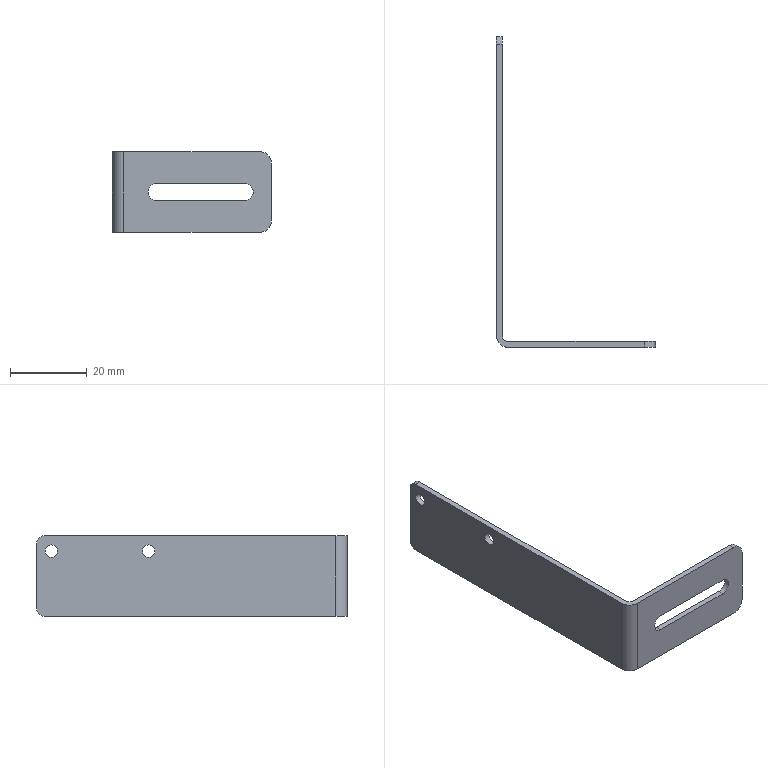Part | STEP file | ROTATION MC_NEW VER-0610_516 | 1 solid | 20 faces | box 41.5 x 81.002 x 21 mm | volume 3574 mm3 | plane 10 | cylinder 10 | commonest cylinder face diameters 6 x3 3.2 x2 4 x2 4.4 x2 3 x1
STEP:
#1=CARTESIAN_POINT('',(-92.489,288.968,-73.528));
#2=VERTEX_POINT('',#1);
#3=CARTESIAN_POINT('',(-115.489,288.968,-73.528));
#4=VERTEX_POINT('',#3);
#5=CARTESIAN_POINT('',(-121.239,288.968,-73.528));
#6=DIRECTION('',(-1.,0.,0.));
#7=VECTOR('',#6,10.);
#8=LINE('',#5,#7);
#9=EDGE_CURVE('',#2,#4,#8,.T.);
#10=ORIENTED_EDGE('',*,*,#9,.F.);
#11=CARTESIAN_POINT('',(-92.489,290.468,-73.528));
#12=VERTEX_POINT('',#11);
#13=CARTESIAN_POINT('',(-92.489,290.468,-73.528));
#14=DIRECTION('',(0.,-1.,0.));
#15=VECTOR('',#14,10.);
#16=LINE('',#13,#15);
#17=EDGE_CURVE('',#12,#2,#16,.T.);
#18=ORIENTED_EDGE('',*,*,#17,.F.);
#19=CARTESIAN_POINT('',(-115.489,290.468,-73.528));
#20=VERTEX_POINT('',#19);
#21=CARTESIAN_POINT('',(-120.489,290.468,-73.528));
#22=DIRECTION('',(1.,0.,0.));
#23=VECTOR('',#22,10.);
#24=LINE('',#21,#23);
#25=EDGE_CURVE('',#20,#12,#24,.T.);
#26=ORIENTED_EDGE('',*,*,#25,.F.);
#27=CARTESIAN_POINT('',(-115.489,290.468,-73.528));
#28=DIRECTION('',(0.,-1.,0.));
#29=VECTOR('',#28,10.);
#30=LINE('',#27,#29);
#31=EDGE_CURVE('',#20,#4,#30,.T.);
#32=ORIENTED_EDGE('',*,*,#31,.T.);
#33=EDGE_LOOP('',(#10,#18,#26,#32));
#34=FACE_OUTER_BOUND('',#33,.T.);
#35=CARTESIAN_POINT('',(-115.489,290.468,-73.528));
#36=DIRECTION('',(0.,0.,-1.));
#37=DIRECTION('',(1.,0.,0.));
#38=AXIS2_PLACEMENT_3D('',#35,#36,#37);
#39=PLANE('',#38);
#40=ADVANCED_FACE('',(#34),#39,.F.);
#41=CARTESIAN_POINT('',(-115.489,288.968,-69.128));
#42=VERTEX_POINT('',#41);
#43=CARTESIAN_POINT('',(-115.489,288.968,-71.328));
#44=DIRECTION('',(0.,1.,0.));
#45=DIRECTION('',(0.,0.,-1.));
#46=AXIS2_PLACEMENT_3D('',#43,#44,#45);
#47=CIRCLE('',#46,2.2);
#48=EDGE_CURVE('',#4,#42,#47,.T.);
#49=ORIENTED_EDGE('',*,*,#48,.F.);
#50=ORIENTED_EDGE('',*,*,#31,.F.);
#51=CARTESIAN_POINT('',(-115.489,290.468,-69.128));
#52=VERTEX_POINT('',#51);
#53=CARTESIAN_POINT('',(-115.489,290.468,-71.328));
#54=DIRECTION('',(0.,-1.,0.));
#55=DIRECTION('',(0.,0.,-1.));
#56=AXIS2_PLACEMENT_3D('',#53,#54,#55);
#57=CIRCLE('',#56,2.2);
#58=EDGE_CURVE('',#52,#20,#57,.T.);
#59=ORIENTED_EDGE('',*,*,#58,.F.);
#60=CARTESIAN_POINT('',(-115.489,290.468,-69.128));
#61=DIRECTION('',(0.,-1.,0.));
#62=VECTOR('',#61,10.);
#63=LINE('',#60,#62);
#64=EDGE_CURVE('',#52,#42,#63,.T.);
#65=ORIENTED_EDGE('',*,*,#64,.T.);
#66=EDGE_LOOP('',(#49,#50,#59,#65));
#67=FACE_OUTER_BOUND('',#66,.T.);
#68=CARTESIAN_POINT('',(-115.489,290.468,-71.328));
#69=DIRECTION('',(0.,-1.,0.));
#70=DIRECTION('',(0.,0.,-1.));
#71=AXIS2_PLACEMENT_3D('',#68,#69,#70);
#72=CYLINDRICAL_SURFACE('',#71,2.2);
#73=ADVANCED_FACE('',(#67),#72,.F.);
#74=CARTESIAN_POINT('',(-92.489,288.968,-69.128));
#75=VERTEX_POINT('',#74);
#76=CARTESIAN_POINT('',(-109.739,288.968,-69.128));
#77=DIRECTION('',(1.,0.,0.));
#78=VECTOR('',#77,10.);
#79=LINE('',#76,#78);
#80=EDGE_CURVE('',#42,#75,#79,.T.);
#81=ORIENTED_EDGE('',*,*,#80,.F.);
#82=ORIENTED_EDGE('',*,*,#64,.F.);
#83=CARTESIAN_POINT('',(-92.489,290.468,-69.128));
#84=VERTEX_POINT('',#83);
#85=CARTESIAN_POINT('',(-108.989,290.468,-69.128));
#86=DIRECTION('',(-1.,0.,0.));
#87=VECTOR('',#86,10.);
#88=LINE('',#85,#87);
#89=EDGE_CURVE('',#84,#52,#88,.T.);
#90=ORIENTED_EDGE('',*,*,#89,.F.);
#91=CARTESIAN_POINT('',(-92.489,290.468,-69.128));
#92=DIRECTION('',(0.,-1.,0.));
#93=VECTOR('',#92,10.);
#94=LINE('',#91,#93);
#95=EDGE_CURVE('',#84,#75,#94,.T.);
#96=ORIENTED_EDGE('',*,*,#95,.T.);
#97=EDGE_LOOP('',(#81,#82,#90,#96));
#98=FACE_OUTER_BOUND('',#97,.T.);
#99=CARTESIAN_POINT('',(-92.489,290.468,-69.128));
#100=DIRECTION('',(0.,0.,1.));
#101=DIRECTION('',(-1.,0.,0.));
#102=AXIS2_PLACEMENT_3D('',#99,#100,#101);
#103=PLANE('',#102);
#104=ADVANCED_FACE('',(#98),#103,.F.);
#105=CARTESIAN_POINT('',(-92.489,288.968,-71.328));
#106=DIRECTION('',(0.,1.,0.));
#107=DIRECTION('',(0.,0.,1.));
#108=AXIS2_PLACEMENT_3D('',#105,#106,#107);
#109=CIRCLE('',#108,2.2);
#110=EDGE_CURVE('',#75,#2,#109,.T.);
#111=ORIENTED_EDGE('',*,*,#110,.F.);
#112=ORIENTED_EDGE('',*,*,#95,.F.);
#113=CARTESIAN_POINT('',(-92.489,290.468,-71.328));
#114=DIRECTION('',(0.,-1.,0.));
#115=DIRECTION('',(0.,0.,1.));
#116=AXIS2_PLACEMENT_3D('',#113,#114,#115);
#117=CIRCLE('',#116,2.2);
#118=EDGE_CURVE('',#12,#84,#117,.T.);
#119=ORIENTED_EDGE('',*,*,#118,.F.);
#120=ORIENTED_EDGE('',*,*,#17,.T.);
#121=EDGE_LOOP('',(#111,#112,#119,#120));
#122=FACE_OUTER_BOUND('',#121,.T.);
#123=CARTESIAN_POINT('',(-92.489,290.468,-71.328));
#124=DIRECTION('',(0.,-1.,0.));
#125=DIRECTION('',(0.,0.,1.));
#126=AXIS2_PLACEMENT_3D('',#123,#124,#125);
#127=CYLINDRICAL_SURFACE('',#126,2.2);
#128=ADVANCED_FACE('',(#122),#127,.F.);
#129=CARTESIAN_POINT('',(-88.489,290.468,-81.828));
#130=VERTEX_POINT('',#129);
#131=CARTESIAN_POINT('',(-85.489,290.468,-78.828));
#132=VERTEX_POINT('',#131);
#133=CARTESIAN_POINT('',(-88.489,290.468,-78.828));
#134=DIRECTION('',(0.,-1.,0.));
#135=DIRECTION('',(0.7071,0.,-0.7071));
#136=AXIS2_PLACEMENT_3D('',#133,#134,#135);
#137=CIRCLE('',#136,3.);
#138=EDGE_CURVE('',#130,#132,#137,.T.);
#139=ORIENTED_EDGE('',*,*,#138,.T.);
#140=CARTESIAN_POINT('',(-85.489,288.968,-78.828));
#141=VERTEX_POINT('',#140);
#142=CARTESIAN_POINT('',(-85.489,386.581,-78.828));
#143=DIRECTION('',(0.,-1.,0.));
#144=VECTOR('',#143,10.);
#145=LINE('',#142,#144);
#146=EDGE_CURVE('',#132,#141,#145,.T.);
#147=ORIENTED_EDGE('',*,*,#146,.T.);
#148=CARTESIAN_POINT('',(-88.489,288.968,-81.828));
#149=VERTEX_POINT('',#148);
#150=CARTESIAN_POINT('',(-88.489,288.968,-78.828));
#151=DIRECTION('',(0.,1.,0.));
#152=DIRECTION('',(0.7071,0.,-0.7071));
#153=AXIS2_PLACEMENT_3D('',#150,#151,#152);
#154=CIRCLE('',#153,3.);
#155=EDGE_CURVE('',#141,#149,#154,.T.);
#156=ORIENTED_EDGE('',*,*,#155,.T.);
#157=CARTESIAN_POINT('',(-88.489,386.581,-81.828));
#158=DIRECTION('',(0.,1.,0.));
#159=VECTOR('',#158,10.);
#160=LINE('',#157,#159);
#161=EDGE_CURVE('',#149,#130,#160,.T.);
#162=ORIENTED_EDGE('',*,*,#161,.T.);
#163=EDGE_LOOP('',(#139,#147,#156,#162));
#164=FACE_OUTER_BOUND('',#163,.T.);
#165=CARTESIAN_POINT('',(-88.489,386.581,-78.828));
#166=DIRECTION('',(0.,1.,0.));
#167=DIRECTION('',(0.7071,0.,-0.7071));
#168=AXIS2_PLACEMENT_3D('',#165,#166,#167);
#169=CYLINDRICAL_SURFACE('',#168,3.);
#170=ADVANCED_FACE('',(#164),#169,.T.);
#171=ORIENTED_EDGE('',*,*,#155,.F.);
#172=CARTESIAN_POINT('',(-85.489,288.968,-63.828));
#173=VERTEX_POINT('',#172);
#174=CARTESIAN_POINT('',(-85.489,288.968,-78.828));
#175=DIRECTION('',(0.,0.,1.));
#176=VECTOR('',#175,15.);
#177=LINE('',#174,#176);
#178=EDGE_CURVE('',#141,#173,#177,.T.);
#179=ORIENTED_EDGE('',*,*,#178,.T.);
#180=CARTESIAN_POINT('',(-88.489,288.968,-60.828));
#181=VERTEX_POINT('',#180);
#182=CARTESIAN_POINT('',(-88.489,288.968,-63.828));
#183=DIRECTION('',(0.,1.,0.));
#184=DIRECTION('',(0.7071,0.,0.7071));
#185=AXIS2_PLACEMENT_3D('',#182,#183,#184);
#186=CIRCLE('',#185,3.);
#187=EDGE_CURVE('',#181,#173,#186,.T.);
#188=ORIENTED_EDGE('',*,*,#187,.F.);
#189=CARTESIAN_POINT('',(-123.989,288.968,-60.828));
#190=VERTEX_POINT('',#189);
#191=CARTESIAN_POINT('',(-123.989,288.968,-60.828));
#192=DIRECTION('',(1.,0.,0.));
#193=VECTOR('',#192,25.5);
#194=LINE('',#191,#193);
#195=EDGE_CURVE('',#190,#181,#194,.T.);
#196=ORIENTED_EDGE('',*,*,#195,.F.);
#197=CARTESIAN_POINT('',(-123.989,288.968,-81.828));
#198=VERTEX_POINT('',#197);
#199=CARTESIAN_POINT('',(-123.989,288.968,-81.828));
#200=DIRECTION('',(0.,0.,1.));
#201=VECTOR('',#200,21.);
#202=LINE('',#199,#201);
#203=EDGE_CURVE('',#198,#190,#202,.T.);
#204=ORIENTED_EDGE('',*,*,#203,.F.);
#205=CARTESIAN_POINT('',(-123.989,288.968,-81.828));
#206=DIRECTION('',(1.,0.,0.));
#207=VECTOR('',#206,25.5);
#208=LINE('',#205,#207);
#209=EDGE_CURVE('',#198,#149,#208,.T.);
#210=ORIENTED_EDGE('',*,*,#209,.T.);
#211=EDGE_LOOP('',(#171,#179,#188,#196,#204,#210));
#212=FACE_OUTER_BOUND('',#211,.T.);
#213=ORIENTED_EDGE('',*,*,#80,.T.);
#214=ORIENTED_EDGE('',*,*,#110,.T.);
#215=ORIENTED_EDGE('',*,*,#9,.T.);
#216=ORIENTED_EDGE('',*,*,#48,.T.);
#217=EDGE_LOOP('',(#213,#214,#215,#216));
#218=FACE_BOUND('',#217,.T.);
#219=CARTESIAN_POINT('',(-126.989,288.968,-71.591));
#220=DIRECTION('',(0.,-1.,0.));
#221=DIRECTION('',(0.,0.,-1.));
#222=AXIS2_PLACEMENT_3D('',#219,#220,#221);
#223=PLANE('',#222);
#224=ADVANCED_FACE('',(#212,#218),#223,.T.);
#225=ORIENTED_EDGE('',*,*,#146,.F.);
#226=CARTESIAN_POINT('',(-85.489,290.468,-63.828));
#227=VERTEX_POINT('',#226);
#228=CARTESIAN_POINT('',(-85.489,290.468,-78.828));
#229=DIRECTION('',(0.,0.,1.));
#230=VECTOR('',#229,15.);
#231=LINE('',#228,#230);
#232=EDGE_CURVE('',#132,#227,#231,.T.);
#233=ORIENTED_EDGE('',*,*,#232,.T.);
#234=CARTESIAN_POINT('',(-85.489,386.581,-63.828));
#235=DIRECTION('',(0.,1.,0.));
#236=VECTOR('',#235,10.);
#237=LINE('',#234,#236);
#238=EDGE_CURVE('',#173,#227,#237,.T.);
#239=ORIENTED_EDGE('',*,*,#238,.F.);
#240=ORIENTED_EDGE('',*,*,#178,.F.);
#241=EDGE_LOOP('',(#225,#233,#239,#240));
#242=FACE_OUTER_BOUND('',#241,.T.);
#243=CARTESIAN_POINT('',(-85.489,422.081,-91.591));
#244=DIRECTION('',(1.,0.,0.));
#245=DIRECTION('',(0.,0.,-1.));
#246=AXIS2_PLACEMENT_3D('',#243,#244,#245);
#247=PLANE('',#246);
#248=ADVANCED_FACE('',(#242),#247,.T.);
#249=CARTESIAN_POINT('',(-88.489,290.468,-60.828));
#250=VERTEX_POINT('',#249);
#251=CARTESIAN_POINT('',(-88.489,290.468,-63.828));
#252=DIRECTION('',(0.,-1.,0.));
#253=DIRECTION('',(0.7071,0.,0.7071));
#254=AXIS2_PLACEMENT_3D('',#251,#252,#253);
#255=CIRCLE('',#254,3.);
#256=EDGE_CURVE('',#227,#250,#255,.T.);
#257=ORIENTED_EDGE('',*,*,#256,.T.);
#258=CARTESIAN_POINT('',(-88.489,386.581,-60.828));
#259=DIRECTION('',(0.,-1.,0.));
#260=VECTOR('',#259,10.);
#261=LINE('',#258,#260);
#262=EDGE_CURVE('',#250,#181,#261,.T.);
#263=ORIENTED_EDGE('',*,*,#262,.T.);
#264=ORIENTED_EDGE('',*,*,#187,.T.);
#265=ORIENTED_EDGE('',*,*,#238,.T.);
#266=EDGE_LOOP('',(#257,#263,#264,#265));
#267=FACE_OUTER_BOUND('',#266,.T.);
#268=CARTESIAN_POINT('',(-88.489,386.581,-63.828));
#269=DIRECTION('',(0.,1.,0.));
#270=DIRECTION('',(0.7071,0.,0.7071));
#271=AXIS2_PLACEMENT_3D('',#268,#269,#270);
#272=CYLINDRICAL_SURFACE('',#271,3.);
#273=ADVANCED_FACE('',(#267),#272,.T.);
#274=ORIENTED_EDGE('',*,*,#161,.F.);
#275=ORIENTED_EDGE('',*,*,#209,.F.);
#276=CARTESIAN_POINT('',(-126.989,291.968,-81.828));
#277=VERTEX_POINT('',#276);
#278=CARTESIAN_POINT('',(-123.989,291.968,-81.828));
#279=DIRECTION('',(0.,0.,1.));
#280=DIRECTION('',(-0.7071,-0.7071,0.));
#281=AXIS2_PLACEMENT_3D('',#278,#279,#280);
#282=CIRCLE('',#281,3.);
#283=EDGE_CURVE('',#277,#198,#282,.T.);
#284=ORIENTED_EDGE('',*,*,#283,.F.);
#285=CARTESIAN_POINT('',(-126.989,367.967,-81.828));
#286=VERTEX_POINT('',#285);
#287=CARTESIAN_POINT('',(-126.989,367.967,-81.828));
#288=DIRECTION('',(0.,-1.,0.));
#289=VECTOR('',#288,75.999);
#290=LINE('',#287,#289);
#291=EDGE_CURVE('',#286,#277,#290,.T.);
#292=ORIENTED_EDGE('',*,*,#291,.F.);
#293=CARTESIAN_POINT('',(-125.489,367.967,-81.828));
#294=VERTEX_POINT('',#293);
#295=CARTESIAN_POINT('',(-126.989,367.967,-81.828));
#296=DIRECTION('',(1.,0.,0.));
#297=VECTOR('',#296,1.5);
#298=LINE('',#295,#297);
#299=EDGE_CURVE('',#286,#294,#298,.T.);
#300=ORIENTED_EDGE('',*,*,#299,.T.);
#301=CARTESIAN_POINT('',(-125.489,291.968,-81.828));
#302=VERTEX_POINT('',#301);
#303=CARTESIAN_POINT('',(-125.489,367.967,-81.828));
#304=DIRECTION('',(0.,-1.,0.));
#305=VECTOR('',#304,75.999);
#306=LINE('',#303,#305);
#307=EDGE_CURVE('',#294,#302,#306,.T.);
#308=ORIENTED_EDGE('',*,*,#307,.T.);
#309=CARTESIAN_POINT('',(-123.989,290.468,-81.828));
#310=VERTEX_POINT('',#309);
#311=CARTESIAN_POINT('',(-123.989,291.968,-81.828));
#312=DIRECTION('',(0.,0.,-1.));
#313=DIRECTION('',(-0.7071,-0.7071,0.));
#314=AXIS2_PLACEMENT_3D('',#311,#312,#313);
#315=CIRCLE('',#314,1.5);
#316=EDGE_CURVE('',#310,#302,#315,.T.);
#317=ORIENTED_EDGE('',*,*,#316,.F.);
#318=CARTESIAN_POINT('',(-98.489,290.468,-81.828));
#319=DIRECTION('',(-1.,0.,0.));
#320=VECTOR('',#319,25.5);
#321=LINE('',#318,#320);
#322=EDGE_CURVE('',#130,#310,#321,.T.);
#323=ORIENTED_EDGE('',*,*,#322,.F.);
#324=EDGE_LOOP('',(#274,#275,#284,#292,#300,#308,#317,#323));
#325=FACE_OUTER_BOUND('',#324,.T.);
#326=CARTESIAN_POINT('',(-126.989,351.081,-81.828));
#327=DIRECTION('',(0.,0.,-1.));
#328=DIRECTION('',(-1.,0.,0.));
#329=AXIS2_PLACEMENT_3D('',#326,#327,#328);
#330=PLANE('',#329);
#331=ADVANCED_FACE('',(#325),#330,.T.);
#332=CARTESIAN_POINT('',(-126.989,367.97,-60.828));
#333=VERTEX_POINT('',#332);
#334=CARTESIAN_POINT('',(-126.989,369.97,-62.829));
#335=VERTEX_POINT('',#334);
#336=CARTESIAN_POINT('',(-126.989,367.97,-62.828));
#337=DIRECTION('',(-1.,0.,0.));
#338=DIRECTION('',(0.,0.,-1.));
#339=AXIS2_PLACEMENT_3D('',#336,#337,#338);
#340=CIRCLE('',#339,2.);
#341=EDGE_CURVE('',#333,#335,#340,.T.);
#342=ORIENTED_EDGE('',*,*,#341,.F.);
#343=CARTESIAN_POINT('',(-125.489,367.97,-60.828));
#344=VERTEX_POINT('',#343);
#345=CARTESIAN_POINT('',(-125.489,367.97,-60.828));
#346=DIRECTION('',(-1.,0.,0.));
#347=VECTOR('',#346,1.5);
#348=LINE('',#345,#347);
#349=EDGE_CURVE('',#344,#333,#348,.T.);
#350=ORIENTED_EDGE('',*,*,#349,.F.);
#351=CARTESIAN_POINT('',(-125.489,369.97,-62.829));
#352=VERTEX_POINT('',#351);
#353=CARTESIAN_POINT('',(-125.489,367.97,-62.828));
#354=DIRECTION('',(1.,0.,0.));
#355=DIRECTION('',(0.,0.,-1.));
#356=AXIS2_PLACEMENT_3D('',#353,#354,#355);
#357=CIRCLE('',#356,2.);
#358=EDGE_CURVE('',#352,#344,#357,.T.);
#359=ORIENTED_EDGE('',*,*,#358,.F.);
#360=CARTESIAN_POINT('',(-126.989,369.97,-62.829));
#361=DIRECTION('',(1.,0.,0.));
#362=VECTOR('',#361,1.5);
#363=LINE('',#360,#362);
#364=EDGE_CURVE('',#335,#352,#363,.T.);
#365=ORIENTED_EDGE('',*,*,#364,.F.);
#366=EDGE_LOOP('',(#342,#350,#359,#365));
#367=FACE_OUTER_BOUND('',#366,.T.);
#368=CARTESIAN_POINT('',(-132.189,367.97,-62.828));
#369=DIRECTION('',(1.,0.,0.));
#370=DIRECTION('',(0.,0.,-1.));
#371=AXIS2_PLACEMENT_3D('',#368,#369,#370);
#372=CYLINDRICAL_SURFACE('',#371,2.);
#373=ADVANCED_FACE('',(#367),#372,.T.);
#374=CARTESIAN_POINT('',(-126.989,369.967,-79.829));
#375=VERTEX_POINT('',#374);
#376=CARTESIAN_POINT('',(-126.989,367.967,-79.828));
#377=DIRECTION('',(-1.,0.,0.));
#378=DIRECTION('',(0.,0.,-1.));
#379=AXIS2_PLACEMENT_3D('',#376,#377,#378);
#380=CIRCLE('',#379,2.);
#381=EDGE_CURVE('',#375,#286,#380,.T.);
#382=ORIENTED_EDGE('',*,*,#381,.F.);
#383=CARTESIAN_POINT('',(-125.489,369.967,-79.829));
#384=VERTEX_POINT('',#383);
#385=CARTESIAN_POINT('',(-125.489,369.967,-79.829));
#386=DIRECTION('',(-1.,0.,0.));
#387=VECTOR('',#386,1.5);
#388=LINE('',#385,#387);
#389=EDGE_CURVE('',#384,#375,#388,.T.);
#390=ORIENTED_EDGE('',*,*,#389,.F.);
#391=CARTESIAN_POINT('',(-125.489,367.967,-79.828));
#392=DIRECTION('',(1.,0.,0.));
#393=DIRECTION('',(0.,0.,-1.));
#394=AXIS2_PLACEMENT_3D('',#391,#392,#393);
#395=CIRCLE('',#394,2.);
#396=EDGE_CURVE('',#294,#384,#395,.T.);
#397=ORIENTED_EDGE('',*,*,#396,.F.);
#398=ORIENTED_EDGE('',*,*,#299,.F.);
#399=EDGE_LOOP('',(#382,#390,#397,#398));
#400=FACE_OUTER_BOUND('',#399,.T.);
#401=CARTESIAN_POINT('',(-126.989,367.967,-79.828));
#402=DIRECTION('',(1.,0.,0.));
#403=DIRECTION('',(0.,0.,-1.));
#404=AXIS2_PLACEMENT_3D('',#401,#402,#403);
#405=CYLINDRICAL_SURFACE('',#404,2.);
#406=ADVANCED_FACE('',(#400),#405,.T.);
#407=CARTESIAN_POINT('',(-126.989,291.968,-60.828));
#408=VERTEX_POINT('',#407);
#409=CARTESIAN_POINT('',(-123.989,291.968,-60.828));
#410=DIRECTION('',(0.,0.,-1.));
#411=DIRECTION('',(-0.7071,-0.7071,0.));
#412=AXIS2_PLACEMENT_3D('',#409,#410,#411);
#413=CIRCLE('',#412,3.);
#414=EDGE_CURVE('',#190,#408,#413,.T.);
#415=ORIENTED_EDGE('',*,*,#414,.T.);
#416=CARTESIAN_POINT('',(-126.989,291.968,-60.828));
#417=DIRECTION('',(0.,0.,-1.));
#418=VECTOR('',#417,21.);
#419=LINE('',#416,#418);
#420=EDGE_CURVE('',#408,#277,#419,.T.);
#421=ORIENTED_EDGE('',*,*,#420,.T.);
#422=ORIENTED_EDGE('',*,*,#283,.T.);
#423=ORIENTED_EDGE('',*,*,#203,.T.);
#424=EDGE_LOOP('',(#415,#421,#422,#423));
#425=FACE_OUTER_BOUND('',#424,.T.);
#426=CARTESIAN_POINT('',(-123.989,291.968,-81.591));
#427=DIRECTION('',(0.,0.,-1.));
#428=DIRECTION('',(-0.7071,-0.7071,0.));
#429=AXIS2_PLACEMENT_3D('',#426,#427,#428);
#430=CYLINDRICAL_SURFACE('',#429,3.);
#431=ADVANCED_FACE('',(#425),#430,.T.);
#432=CARTESIAN_POINT('',(-125.489,340.774,-66.428));
#433=VERTEX_POINT('',#432);
#434=CARTESIAN_POINT('',(-125.489,340.774,-64.828));
#435=DIRECTION('',(1.,0.,0.));
#436=DIRECTION('',(0.,0.,-1.));
#437=AXIS2_PLACEMENT_3D('',#434,#435,#436);
#438=CIRCLE('',#437,1.6);
#439=EDGE_CURVE('',#433,#433,#438,.T.);
#440=ORIENTED_EDGE('',*,*,#439,.T.);
#441=CARTESIAN_POINT('',(-126.989,340.774,-66.428));
#442=VERTEX_POINT('',#441);
#443=CARTESIAN_POINT('',(-132.189,340.774,-66.428));
#444=DIRECTION('',(-1.,0.,0.));
#445=VECTOR('',#444,1.6);
#446=LINE('',#443,#445);
#447=EDGE_CURVE('',#433,#442,#446,.T.);
#448=ORIENTED_EDGE('',*,*,#447,.T.);
#449=CARTESIAN_POINT('',(-126.989,340.774,-64.828));
#450=DIRECTION('',(-1.,0.,0.));
#451=DIRECTION('',(0.,0.,-1.));
#452=AXIS2_PLACEMENT_3D('',#449,#450,#451);
#453=CIRCLE('',#452,1.6);
#454=EDGE_CURVE('',#442,#442,#453,.T.);
#455=ORIENTED_EDGE('',*,*,#454,.T.);
#456=ORIENTED_EDGE('',*,*,#447,.F.);
#457=EDGE_LOOP('',(#440,#448,#455,#456));
#458=FACE_OUTER_BOUND('',#457,.T.);
#459=CARTESIAN_POINT('',(-132.189,340.774,-64.828));
#460=DIRECTION('',(-1.,0.,0.));
#461=DIRECTION('',(0.,0.,1.));
#462=AXIS2_PLACEMENT_3D('',#459,#460,#461);
#463=CYLINDRICAL_SURFACE('',#462,1.6);
#464=ADVANCED_FACE('',(#458),#463,.F.);
#465=CARTESIAN_POINT('',(-125.489,366.174,-66.428));
#466=VERTEX_POINT('',#465);
#467=CARTESIAN_POINT('',(-125.489,366.174,-64.828));
#468=DIRECTION('',(1.,0.,0.));
#469=DIRECTION('',(0.,0.,-1.));
#470=AXIS2_PLACEMENT_3D('',#467,#468,#469);
#471=CIRCLE('',#470,1.6);
#472=EDGE_CURVE('',#466,#466,#471,.T.);
#473=ORIENTED_EDGE('',*,*,#472,.T.);
#474=CARTESIAN_POINT('',(-126.989,366.174,-66.428));
#475=VERTEX_POINT('',#474);
#476=CARTESIAN_POINT('',(-132.189,366.174,-66.428));
#477=DIRECTION('',(-1.,0.,0.));
#478=VECTOR('',#477,1.6);
#479=LINE('',#476,#478);
#480=EDGE_CURVE('',#466,#475,#479,.T.);
#481=ORIENTED_EDGE('',*,*,#480,.T.);
#482=CARTESIAN_POINT('',(-126.989,366.174,-64.828));
#483=DIRECTION('',(-1.,0.,0.));
#484=DIRECTION('',(0.,0.,-1.));
#485=AXIS2_PLACEMENT_3D('',#482,#483,#484);
#486=CIRCLE('',#485,1.6);
#487=EDGE_CURVE('',#475,#475,#486,.T.);
#488=ORIENTED_EDGE('',*,*,#487,.T.);
#489=ORIENTED_EDGE('',*,*,#480,.F.);
#490=EDGE_LOOP('',(#473,#481,#488,#489));
#491=FACE_OUTER_BOUND('',#490,.T.);
#492=CARTESIAN_POINT('',(-132.189,366.174,-64.828));
#493=DIRECTION('',(-1.,0.,0.));
#494=DIRECTION('',(0.,0.,1.));
#495=AXIS2_PLACEMENT_3D('',#492,#493,#494);
#496=CYLINDRICAL_SURFACE('',#495,1.6);
#497=ADVANCED_FACE('',(#491),#496,.F.);
#498=CARTESIAN_POINT('',(-125.489,291.968,-60.828));
#499=VERTEX_POINT('',#498);
#500=CARTESIAN_POINT('',(-123.989,290.468,-60.828));
#501=VERTEX_POINT('',#500);
#502=CARTESIAN_POINT('',(-123.989,291.968,-60.828));
#503=DIRECTION('',(0.,0.,1.));
#504=DIRECTION('',(-0.7071,-0.7071,0.));
#505=AXIS2_PLACEMENT_3D('',#502,#503,#504);
#506=CIRCLE('',#505,1.5);
#507=EDGE_CURVE('',#499,#501,#506,.T.);
#508=ORIENTED_EDGE('',*,*,#507,.T.);
#509=CARTESIAN_POINT('',(-123.989,290.468,-60.828));
#510=DIRECTION('',(0.,0.,-1.));
#511=VECTOR('',#510,21.);
#512=LINE('',#509,#511);
#513=EDGE_CURVE('',#501,#310,#512,.T.);
#514=ORIENTED_EDGE('',*,*,#513,.T.);
#515=ORIENTED_EDGE('',*,*,#316,.T.);
#516=CARTESIAN_POINT('',(-125.489,291.968,-81.828));
#517=DIRECTION('',(0.,0.,1.));
#518=VECTOR('',#517,21.);
#519=LINE('',#516,#518);
#520=EDGE_CURVE('',#302,#499,#519,.T.);
#521=ORIENTED_EDGE('',*,*,#520,.T.);
#522=EDGE_LOOP('',(#508,#514,#515,#521));
#523=FACE_OUTER_BOUND('',#522,.T.);
#524=CARTESIAN_POINT('',(-123.989,291.968,-81.591));
#525=DIRECTION('',(0.,0.,-1.));
#526=DIRECTION('',(-0.7071,-0.7071,0.));
#527=AXIS2_PLACEMENT_3D('',#524,#525,#526);
#528=CYLINDRICAL_SURFACE('',#527,1.5);
#529=ADVANCED_FACE('',(#523),#528,.F.);
#530=CARTESIAN_POINT('',(-126.989,369.97,-62.829));
#531=DIRECTION('',(0.,-0.0001883,-1.));
#532=VECTOR('',#531,17.);
#533=LINE('',#530,#532);
#534=EDGE_CURVE('',#335,#375,#533,.T.);
#535=ORIENTED_EDGE('',*,*,#534,.T.);
#536=ORIENTED_EDGE('',*,*,#381,.T.);
#537=ORIENTED_EDGE('',*,*,#291,.T.);
#538=ORIENTED_EDGE('',*,*,#420,.F.);
#539=CARTESIAN_POINT('',(-126.989,291.968,-60.828));
#540=DIRECTION('',(0.,1.,0.));
#541=VECTOR('',#540,76.002);
#542=LINE('',#539,#541);
#543=EDGE_CURVE('',#408,#333,#542,.T.);
#544=ORIENTED_EDGE('',*,*,#543,.T.);
#545=ORIENTED_EDGE('',*,*,#341,.T.);
#546=EDGE_LOOP('',(#535,#536,#537,#538,#544,#545));
#547=FACE_OUTER_BOUND('',#546,.T.);
#548=ORIENTED_EDGE('',*,*,#454,.F.);
#549=EDGE_LOOP('',(#548));
#550=FACE_BOUND('',#549,.T.);
#551=ORIENTED_EDGE('',*,*,#487,.F.);
#552=EDGE_LOOP('',(#551));
#553=FACE_BOUND('',#552,.T.);
#554=CARTESIAN_POINT('',(-126.989,422.081,-91.591));
#555=DIRECTION('',(1.,0.,0.));
#556=DIRECTION('',(0.,0.,-1.));
#557=AXIS2_PLACEMENT_3D('',#554,#555,#556);
#558=PLANE('',#557);
#559=ADVANCED_FACE('',(#547,#550,#553),#558,.F.);
#560=ORIENTED_EDGE('',*,*,#262,.F.);
#561=CARTESIAN_POINT('',(-123.989,290.468,-60.828));
#562=DIRECTION('',(1.,0.,0.));
#563=VECTOR('',#562,25.5);
#564=LINE('',#561,#563);
#565=EDGE_CURVE('',#501,#250,#564,.T.);
#566=ORIENTED_EDGE('',*,*,#565,.F.);
#567=ORIENTED_EDGE('',*,*,#507,.F.);
#568=CARTESIAN_POINT('',(-125.489,291.968,-60.828));
#569=DIRECTION('',(0.,1.,0.));
#570=VECTOR('',#569,76.002);
#571=LINE('',#568,#570);
#572=EDGE_CURVE('',#499,#344,#571,.T.);
#573=ORIENTED_EDGE('',*,*,#572,.T.);
#574=ORIENTED_EDGE('',*,*,#349,.T.);
#575=ORIENTED_EDGE('',*,*,#543,.F.);
#576=ORIENTED_EDGE('',*,*,#414,.F.);
#577=ORIENTED_EDGE('',*,*,#195,.T.);
#578=EDGE_LOOP('',(#560,#566,#567,#573,#574,#575,#576,#577));
#579=FACE_OUTER_BOUND('',#578,.T.);
#580=CARTESIAN_POINT('',(-126.989,351.081,-60.828));
#581=DIRECTION('',(0.,0.,1.));
#582=DIRECTION('',(1.,0.,0.));
#583=AXIS2_PLACEMENT_3D('',#580,#581,#582);
#584=PLANE('',#583);
#585=ADVANCED_FACE('',(#579),#584,.T.);
#586=ORIENTED_EDGE('',*,*,#307,.F.);
#587=ORIENTED_EDGE('',*,*,#396,.T.);
#588=CARTESIAN_POINT('',(-125.489,369.967,-79.829));
#589=DIRECTION('',(0.,0.0001883,1.));
#590=VECTOR('',#589,17.);
#591=LINE('',#588,#590);
#592=EDGE_CURVE('',#384,#352,#591,.T.);
#593=ORIENTED_EDGE('',*,*,#592,.T.);
#594=ORIENTED_EDGE('',*,*,#358,.T.);
#595=ORIENTED_EDGE('',*,*,#572,.F.);
#596=ORIENTED_EDGE('',*,*,#520,.F.);
#597=EDGE_LOOP('',(#586,#587,#593,#594,#595,#596));
#598=FACE_OUTER_BOUND('',#597,.T.);
#599=ORIENTED_EDGE('',*,*,#439,.F.);
#600=EDGE_LOOP('',(#599));
#601=FACE_BOUND('',#600,.T.);
#602=ORIENTED_EDGE('',*,*,#472,.F.);
#603=EDGE_LOOP('',(#602));
#604=FACE_BOUND('',#603,.T.);
#605=CARTESIAN_POINT('',(-125.489,422.081,-91.591));
#606=DIRECTION('',(1.,0.,0.));
#607=DIRECTION('',(0.,0.,-1.));
#608=AXIS2_PLACEMENT_3D('',#605,#606,#607);
#609=PLANE('',#608);
#610=ADVANCED_FACE('',(#598,#601,#604),#609,.T.);
#611=ORIENTED_EDGE('',*,*,#592,.F.);
#612=ORIENTED_EDGE('',*,*,#389,.T.);
#613=ORIENTED_EDGE('',*,*,#534,.F.);
#614=ORIENTED_EDGE('',*,*,#364,.T.);
#615=EDGE_LOOP('',(#611,#612,#613,#614));
#616=FACE_OUTER_BOUND('',#615,.T.);
#617=CARTESIAN_POINT('',(-132.189,369.968,-73.329));
#618=DIRECTION('',(0.,1.,-0.0001883));
#619=DIRECTION('',(0.,0.0001883,1.));
#620=AXIS2_PLACEMENT_3D('',#617,#618,#619);
#621=PLANE('',#620);
#622=ADVANCED_FACE('',(#616),#621,.T.);
#623=ORIENTED_EDGE('',*,*,#138,.F.);
#624=ORIENTED_EDGE('',*,*,#322,.T.);
#625=ORIENTED_EDGE('',*,*,#513,.F.);
#626=ORIENTED_EDGE('',*,*,#565,.T.);
#627=ORIENTED_EDGE('',*,*,#256,.F.);
#628=ORIENTED_EDGE('',*,*,#232,.F.);
#629=EDGE_LOOP('',(#623,#624,#625,#626,#627,#628));
#630=FACE_OUTER_BOUND('',#629,.T.);
#631=ORIENTED_EDGE('',*,*,#89,.T.);
#632=ORIENTED_EDGE('',*,*,#58,.T.);
#633=ORIENTED_EDGE('',*,*,#25,.T.);
#634=ORIENTED_EDGE('',*,*,#118,.T.);
#635=EDGE_LOOP('',(#631,#632,#633,#634));
#636=FACE_BOUND('',#635,.T.);
#637=CARTESIAN_POINT('',(-125.489,290.468,-71.591));
#638=DIRECTION('',(0.,1.,0.));
#639=DIRECTION('',(0.,0.,1.));
#640=AXIS2_PLACEMENT_3D('',#637,#638,#639);
#641=PLANE('',#640);
#642=ADVANCED_FACE('',(#630,#636),#641,.T.);
#643=CLOSED_SHELL('',(#40,#73,#104,#128,#170,#224,#248,#273,#331,#373,#406,#431,#464,#497,#529,#559,#585,#610,#622,#642));
#644=MANIFOLD_SOLID_BREP('',#643);
#645=(LENGTH_UNIT()NAMED_UNIT(*)SI_UNIT(.MILLI.,.METRE.));
#646=UNCERTAINTY_MEASURE_WITH_UNIT(LENGTH_MEASURE(0.01),#645,'','');
#647=(NAMED_UNIT(*)PLANE_ANGLE_UNIT()SI_UNIT($,.RADIAN.));
#648=(NAMED_UNIT(*)SI_UNIT($,.STERADIAN.)SOLID_ANGLE_UNIT());
#649=(GEOMETRIC_REPRESENTATION_CONTEXT(3)GLOBAL_UNCERTAINTY_ASSIGNED_CONTEXT((#646))GLOBAL_UNIT_ASSIGNED_CONTEXT((#645,#647,#648))REPRESENTATION_CONTEXT('',''));
#650=ADVANCED_BREP_SHAPE_REPRESENTATION('',(#644),#649);